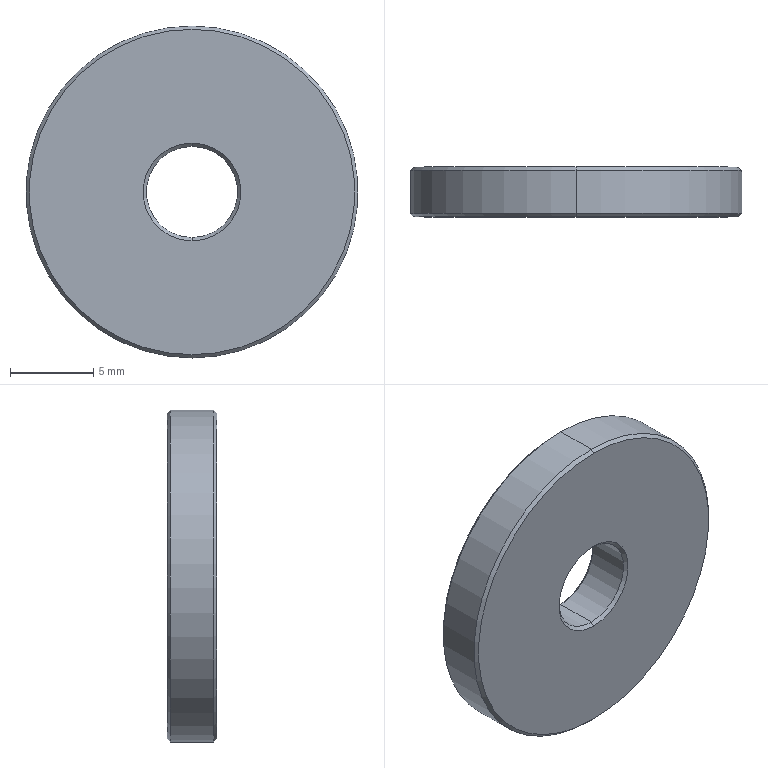Part | STEP file | 1 solid | 14 faces | box 20 x 3 x 20 mm | volume 867.998 mm3 | cone 8 | cylinder 4 | plane 2 | commonest cylinder face diameters 5.5 x2 20 x2
STEP:
#1=CARTESIAN_POINT('',(0.,0.,0.));
#2=DIRECTION('',(0.,0.,1.));
#3=DIRECTION('',(1.,0.,0.));
#4=AXIS2_PLACEMENT_3D('',#1,#2,#3);
#5=CARTESIAN_POINT('',(0.,2.8,2.75));
#6=VERTEX_POINT('',#5);
#7=CARTESIAN_POINT('',(0.,3.,2.95));
#8=VERTEX_POINT('',#7);
#9=CARTESIAN_POINT('',(0.,2.8,2.75));
#10=DIRECTION('',(0.,0.7071,0.7071));
#11=VECTOR('',#10,1.);
#12=LINE('',#9,#11);
#13=CARTESIAN_POINT('',(0.,2.8,0.));
#14=DIRECTION('',(0.,1.,0.));
#15=DIRECTION('',(0.,0.,1.));
#16=AXIS2_PLACEMENT_3D('',#13,#14,#15);
#17=CONICAL_SURFACE('',#16,2.75,0.7854);
#18=CARTESIAN_POINT('',(6.283,0.));
#19=DIRECTION('',(0.,1.));
#20=VECTOR('',#19,1.);
#21=LINE('',#18,#20);
#22=(GEOMETRIC_REPRESENTATION_CONTEXT(2)PARAMETRIC_REPRESENTATION_CONTEXT()REPRESENTATION_CONTEXT('',''));
#23=DEFINITIONAL_REPRESENTATION('',(#21),#22);
#24=PCURVE('',#17,#23);
#25=CARTESIAN_POINT('',(0.,2.8,0.));
#26=DIRECTION('',(0.,1.,0.));
#27=DIRECTION('',(0.,0.,1.));
#28=AXIS2_PLACEMENT_3D('',#25,#26,#27);
#29=CONICAL_SURFACE('',#28,2.75,0.7854);
#30=CARTESIAN_POINT('',(0.,0.));
#31=DIRECTION('',(0.,1.));
#32=VECTOR('',#31,1.);
#33=LINE('',#30,#32);
#34=(GEOMETRIC_REPRESENTATION_CONTEXT(2)PARAMETRIC_REPRESENTATION_CONTEXT()REPRESENTATION_CONTEXT('',''));
#35=DEFINITIONAL_REPRESENTATION('',(#33),#34);
#36=PCURVE('',#29,#35);
#37=SURFACE_CURVE('',#12,(#24,#36),.PCURVE_S1.);
#38=EDGE_CURVE('',#6,#8,#37,.T.);
#39=ORIENTED_EDGE('',*,*,#38,.T.);
#40=CARTESIAN_POINT('',(0.,3.,-2.95));
#41=VERTEX_POINT('',#40);
#42=CARTESIAN_POINT('',(0.,3.,0.));
#43=DIRECTION('',(0.,-1.,0.));
#44=DIRECTION('',(0.,0.,1.));
#45=AXIS2_PLACEMENT_3D('',#42,#43,#44);
#46=CIRCLE('',#45,2.95);
#47=CARTESIAN_POINT('',(6.283,0.2));
#48=DIRECTION('',(-1.,0.));
#49=VECTOR('',#48,1.);
#50=LINE('',#47,#49);
#51=(GEOMETRIC_REPRESENTATION_CONTEXT(2)PARAMETRIC_REPRESENTATION_CONTEXT()REPRESENTATION_CONTEXT('',''));
#52=DEFINITIONAL_REPRESENTATION('',(#50),#51);
#53=PCURVE('',#17,#52);
#54=CARTESIAN_POINT('',(0.,3.,0.));
#55=DIRECTION('',(0.,1.,0.));
#56=DIRECTION('',(0.,0.,1.));
#57=AXIS2_PLACEMENT_3D('',#54,#55,#56);
#58=PLANE('',#57);
#59=CARTESIAN_POINT('',(2.95,0.));
#60=CARTESIAN_POINT('',(2.95,-5.11));
#61=CARTESIAN_POINT('',(-1.475,-2.555));
#62=CARTESIAN_POINT('',(-5.9,0.));
#63=CARTESIAN_POINT('',(-1.475,2.555));
#64=CARTESIAN_POINT('',(2.95,5.11));
#65=CARTESIAN_POINT('',(2.95,0.));
#66=(BOUNDED_CURVE()B_SPLINE_CURVE(2,(#59,#60,#61,#62,#63,#64,#65),.UNSPECIFIED.,.T.,.F.)B_SPLINE_CURVE_WITH_KNOTS((1,2,2,2,2,1),(-2.094,0.,2.094,4.189,6.283,8.378),.UNSPECIFIED.)CURVE()GEOMETRIC_REPRESENTATION_ITEM()RATIONAL_B_SPLINE_CURVE((1.,0.5,1.,0.5,1.,0.5,1.))REPRESENTATION_ITEM(''));
#67=(GEOMETRIC_REPRESENTATION_CONTEXT(2)PARAMETRIC_REPRESENTATION_CONTEXT()REPRESENTATION_CONTEXT('',''));
#68=DEFINITIONAL_REPRESENTATION('',(#66),#67);
#69=PCURVE('',#58,#68);
#70=SURFACE_CURVE('',#46,(#53,#69),.PCURVE_S1.);
#71=EDGE_CURVE('',#8,#41,#70,.T.);
#72=ORIENTED_EDGE('',*,*,#71,.T.);
#73=CARTESIAN_POINT('',(0.,2.8,-2.75));
#74=VERTEX_POINT('',#73);
#75=CARTESIAN_POINT('',(0.,2.8,-2.75));
#76=DIRECTION('',(0.,0.7071,-0.7071));
#77=VECTOR('',#76,1.);
#78=LINE('',#75,#77);
#79=CARTESIAN_POINT('',(3.142,0.));
#80=DIRECTION('',(0.,1.));
#81=VECTOR('',#80,1.);
#82=LINE('',#79,#81);
#83=(GEOMETRIC_REPRESENTATION_CONTEXT(2)PARAMETRIC_REPRESENTATION_CONTEXT()REPRESENTATION_CONTEXT('',''));
#84=DEFINITIONAL_REPRESENTATION('',(#82),#83);
#85=PCURVE('',#17,#84);
#86=CARTESIAN_POINT('',(3.142,0.));
#87=DIRECTION('',(0.,1.));
#88=VECTOR('',#87,1.);
#89=LINE('',#86,#88);
#90=(GEOMETRIC_REPRESENTATION_CONTEXT(2)PARAMETRIC_REPRESENTATION_CONTEXT()REPRESENTATION_CONTEXT('',''));
#91=DEFINITIONAL_REPRESENTATION('',(#89),#90);
#92=PCURVE('',#29,#91);
#93=SURFACE_CURVE('',#78,(#85,#92),.PCURVE_S1.);
#94=EDGE_CURVE('',#74,#41,#93,.T.);
#95=ORIENTED_EDGE('',*,*,#94,.F.);
#96=CARTESIAN_POINT('',(0.,2.8,0.));
#97=DIRECTION('',(0.,1.,0.));
#98=DIRECTION('',(0.,0.,1.));
#99=AXIS2_PLACEMENT_3D('',#96,#97,#98);
#100=CIRCLE('',#99,2.75);
#101=CARTESIAN_POINT('',(0.,0.));
#102=DIRECTION('',(1.,0.));
#103=VECTOR('',#102,1.);
#104=LINE('',#101,#103);
#105=(GEOMETRIC_REPRESENTATION_CONTEXT(2)PARAMETRIC_REPRESENTATION_CONTEXT()REPRESENTATION_CONTEXT('',''));
#106=DEFINITIONAL_REPRESENTATION('',(#104),#105);
#107=PCURVE('',#17,#106);
#108=CARTESIAN_POINT('',(0.,3.,0.));
#109=DIRECTION('',(0.,-1.,0.));
#110=DIRECTION('',(0.,0.,-1.));
#111=AXIS2_PLACEMENT_3D('',#108,#109,#110);
#112=CYLINDRICAL_SURFACE('',#111,2.75);
#113=CARTESIAN_POINT('',(9.425,0.2));
#114=DIRECTION('',(-1.,0.));
#115=VECTOR('',#114,1.);
#116=LINE('',#113,#115);
#117=(GEOMETRIC_REPRESENTATION_CONTEXT(2)PARAMETRIC_REPRESENTATION_CONTEXT()REPRESENTATION_CONTEXT('',''));
#118=DEFINITIONAL_REPRESENTATION('',(#116),#117);
#119=PCURVE('',#112,#118);
#120=SURFACE_CURVE('',#100,(#107,#119),.PCURVE_S1.);
#121=EDGE_CURVE('',#74,#6,#120,.T.);
#122=ORIENTED_EDGE('',*,*,#121,.T.);
#123=EDGE_LOOP('',(#39,#72,#95,#122));
#124=FACE_BOUND('',#123,.F.);
#125=ADVANCED_FACE('',(#124),#17,.F.);
#126=CARTESIAN_POINT('',(0.,0.2,-2.75));
#127=VERTEX_POINT('',#126);
#128=CARTESIAN_POINT('',(0.,0.,-2.95));
#129=VERTEX_POINT('',#128);
#130=CARTESIAN_POINT('',(0.,0.,-2.95));
#131=DIRECTION('',(0.,-0.7071,-0.7071));
#132=VECTOR('',#131,1.);
#133=LINE('',#130,#132);
#134=CARTESIAN_POINT('',(0.,0.,0.));
#135=DIRECTION('',(0.,-1.,0.));
#136=DIRECTION('',(0.,0.,-1.));
#137=AXIS2_PLACEMENT_3D('',#134,#135,#136);
#138=CONICAL_SURFACE('',#137,2.95,0.7854);
#139=CARTESIAN_POINT('',(6.283,0.));
#140=DIRECTION('',(0.,1.));
#141=VECTOR('',#140,1.);
#142=LINE('',#139,#141);
#143=(GEOMETRIC_REPRESENTATION_CONTEXT(2)PARAMETRIC_REPRESENTATION_CONTEXT()REPRESENTATION_CONTEXT('',''));
#144=DEFINITIONAL_REPRESENTATION('',(#142),#143);
#145=PCURVE('',#138,#144);
#146=CARTESIAN_POINT('',(0.,0.,0.));
#147=DIRECTION('',(0.,-1.,0.));
#148=DIRECTION('',(0.,0.,-1.));
#149=AXIS2_PLACEMENT_3D('',#146,#147,#148);
#150=CONICAL_SURFACE('',#149,2.95,0.7854);
#151=CARTESIAN_POINT('',(0.,0.));
#152=DIRECTION('',(0.,1.));
#153=VECTOR('',#152,1.);
#154=LINE('',#151,#153);
#155=(GEOMETRIC_REPRESENTATION_CONTEXT(2)PARAMETRIC_REPRESENTATION_CONTEXT()REPRESENTATION_CONTEXT('',''));
#156=DEFINITIONAL_REPRESENTATION('',(#154),#155);
#157=PCURVE('',#150,#156);
#158=SURFACE_CURVE('',#133,(#145,#157),.PCURVE_S1.);
#159=EDGE_CURVE('',#127,#129,#158,.T.);
#160=ORIENTED_EDGE('',*,*,#159,.T.);
#161=CARTESIAN_POINT('',(0.,0.,2.95));
#162=VERTEX_POINT('',#161);
#163=CARTESIAN_POINT('',(0.,0.,0.));
#164=DIRECTION('',(0.,1.,0.));
#165=DIRECTION('',(0.,0.,1.));
#166=AXIS2_PLACEMENT_3D('',#163,#164,#165);
#167=CIRCLE('',#166,2.95);
#168=CARTESIAN_POINT('',(9.425,0.));
#169=DIRECTION('',(-1.,0.));
#170=VECTOR('',#169,1.);
#171=LINE('',#168,#170);
#172=(GEOMETRIC_REPRESENTATION_CONTEXT(2)PARAMETRIC_REPRESENTATION_CONTEXT()REPRESENTATION_CONTEXT('',''));
#173=DEFINITIONAL_REPRESENTATION('',(#171),#172);
#174=PCURVE('',#138,#173);
#175=CARTESIAN_POINT('',(0.,0.,0.));
#176=DIRECTION('',(0.,1.,0.));
#177=DIRECTION('',(0.,0.,1.));
#178=AXIS2_PLACEMENT_3D('',#175,#176,#177);
#179=PLANE('',#178);
#180=CARTESIAN_POINT('',(0.,0.));
#181=DIRECTION('',(1.,0.));
#182=AXIS2_PLACEMENT_2D('',#180,#181);
#183=CIRCLE('',#182,2.95);
#184=(GEOMETRIC_REPRESENTATION_CONTEXT(2)PARAMETRIC_REPRESENTATION_CONTEXT()REPRESENTATION_CONTEXT('',''));
#185=DEFINITIONAL_REPRESENTATION('',(#183),#184);
#186=PCURVE('',#179,#185);
#187=SURFACE_CURVE('',#167,(#174,#186),.PCURVE_S1.);
#188=EDGE_CURVE('',#129,#162,#187,.T.);
#189=ORIENTED_EDGE('',*,*,#188,.T.);
#190=CARTESIAN_POINT('',(0.,0.2,2.75));
#191=VERTEX_POINT('',#190);
#192=CARTESIAN_POINT('',(0.,0.,2.95));
#193=DIRECTION('',(0.,-0.7071,0.7071));
#194=VECTOR('',#193,1.);
#195=LINE('',#192,#194);
#196=CARTESIAN_POINT('',(3.142,0.));
#197=DIRECTION('',(0.,1.));
#198=VECTOR('',#197,1.);
#199=LINE('',#196,#198);
#200=(GEOMETRIC_REPRESENTATION_CONTEXT(2)PARAMETRIC_REPRESENTATION_CONTEXT()REPRESENTATION_CONTEXT('',''));
#201=DEFINITIONAL_REPRESENTATION('',(#199),#200);
#202=PCURVE('',#138,#201);
#203=CARTESIAN_POINT('',(3.142,0.));
#204=DIRECTION('',(0.,1.));
#205=VECTOR('',#204,1.);
#206=LINE('',#203,#205);
#207=(GEOMETRIC_REPRESENTATION_CONTEXT(2)PARAMETRIC_REPRESENTATION_CONTEXT()REPRESENTATION_CONTEXT('',''));
#208=DEFINITIONAL_REPRESENTATION('',(#206),#207);
#209=PCURVE('',#150,#208);
#210=SURFACE_CURVE('',#195,(#202,#209),.PCURVE_S1.);
#211=EDGE_CURVE('',#191,#162,#210,.T.);
#212=ORIENTED_EDGE('',*,*,#211,.F.);
#213=CARTESIAN_POINT('',(0.,0.2,0.));
#214=DIRECTION('',(0.,-1.,0.));
#215=DIRECTION('',(0.,0.,1.));
#216=AXIS2_PLACEMENT_3D('',#213,#214,#215);
#217=CIRCLE('',#216,2.75);
#218=CARTESIAN_POINT('',(3.142,-0.2));
#219=DIRECTION('',(1.,0.));
#220=VECTOR('',#219,1.);
#221=LINE('',#218,#220);
#222=(GEOMETRIC_REPRESENTATION_CONTEXT(2)PARAMETRIC_REPRESENTATION_CONTEXT()REPRESENTATION_CONTEXT('',''));
#223=DEFINITIONAL_REPRESENTATION('',(#221),#222);
#224=PCURVE('',#138,#223);
#225=CARTESIAN_POINT('',(3.142,2.8));
#226=DIRECTION('',(1.,0.));
#227=VECTOR('',#226,1.);
#228=LINE('',#225,#227);
#229=(GEOMETRIC_REPRESENTATION_CONTEXT(2)PARAMETRIC_REPRESENTATION_CONTEXT()REPRESENTATION_CONTEXT('',''));
#230=DEFINITIONAL_REPRESENTATION('',(#228),#229);
#231=PCURVE('',#112,#230);
#232=SURFACE_CURVE('',#217,(#224,#231),.PCURVE_S1.);
#233=EDGE_CURVE('',#191,#127,#232,.T.);
#234=ORIENTED_EDGE('',*,*,#233,.T.);
#235=EDGE_LOOP('',(#160,#189,#212,#234));
#236=FACE_BOUND('',#235,.F.);
#237=ADVANCED_FACE('',(#236),#138,.F.);
#238=CARTESIAN_POINT('',(0.,3.,9.8));
#239=VERTEX_POINT('',#238);
#240=CARTESIAN_POINT('',(0.,3.,-9.8));
#241=VERTEX_POINT('',#240);
#242=CARTESIAN_POINT('',(0.,3.,0.));
#243=DIRECTION('',(0.,1.,0.));
#244=DIRECTION('',(0.,0.,1.));
#245=AXIS2_PLACEMENT_3D('',#242,#243,#244);
#246=CIRCLE('',#245,9.8);
#247=CARTESIAN_POINT('',(0.,3.,0.));
#248=DIRECTION('',(0.,-1.,0.));
#249=DIRECTION('',(0.,0.,-1.));
#250=AXIS2_PLACEMENT_3D('',#247,#248,#249);
#251=CONICAL_SURFACE('',#250,9.8,0.7854);
#252=CARTESIAN_POINT('',(3.142,0.));
#253=DIRECTION('',(-1.,0.));
#254=VECTOR('',#253,1.);
#255=LINE('',#252,#254);
#256=(GEOMETRIC_REPRESENTATION_CONTEXT(2)PARAMETRIC_REPRESENTATION_CONTEXT()REPRESENTATION_CONTEXT('',''));
#257=DEFINITIONAL_REPRESENTATION('',(#255),#256);
#258=PCURVE('',#251,#257);
#259=CARTESIAN_POINT('',(0.,0.));
#260=DIRECTION('',(1.,0.));
#261=AXIS2_PLACEMENT_2D('',#259,#260);
#262=CIRCLE('',#261,9.8);
#263=(GEOMETRIC_REPRESENTATION_CONTEXT(2)PARAMETRIC_REPRESENTATION_CONTEXT()REPRESENTATION_CONTEXT('',''));
#264=DEFINITIONAL_REPRESENTATION('',(#262),#263);
#265=PCURVE('',#58,#264);
#266=SURFACE_CURVE('',#246,(#258,#265),.PCURVE_S1.);
#267=EDGE_CURVE('',#239,#241,#266,.T.);
#268=ORIENTED_EDGE('',*,*,#267,.F.);
#269=CARTESIAN_POINT('',(0.,2.8,10.));
#270=VERTEX_POINT('',#269);
#271=CARTESIAN_POINT('',(0.,3.,9.8));
#272=DIRECTION('',(0.,-0.7071,0.7071));
#273=VECTOR('',#272,1.);
#274=LINE('',#271,#273);
#275=CARTESIAN_POINT('',(3.142,0.));
#276=DIRECTION('',(0.,1.));
#277=VECTOR('',#276,1.);
#278=LINE('',#275,#277);
#279=(GEOMETRIC_REPRESENTATION_CONTEXT(2)PARAMETRIC_REPRESENTATION_CONTEXT()REPRESENTATION_CONTEXT('',''));
#280=DEFINITIONAL_REPRESENTATION('',(#278),#279);
#281=PCURVE('',#251,#280);
#282=CARTESIAN_POINT('',(0.,3.,0.));
#283=DIRECTION('',(0.,-1.,0.));
#284=DIRECTION('',(0.,0.,-1.));
#285=AXIS2_PLACEMENT_3D('',#282,#283,#284);
#286=CONICAL_SURFACE('',#285,9.8,0.7854);
#287=CARTESIAN_POINT('',(3.142,0.));
#288=DIRECTION('',(0.,1.));
#289=VECTOR('',#288,1.);
#290=LINE('',#287,#289);
#291=(GEOMETRIC_REPRESENTATION_CONTEXT(2)PARAMETRIC_REPRESENTATION_CONTEXT()REPRESENTATION_CONTEXT('',''));
#292=DEFINITIONAL_REPRESENTATION('',(#290),#291);
#293=PCURVE('',#286,#292);
#294=SURFACE_CURVE('',#274,(#281,#293),.PCURVE_S1.);
#295=EDGE_CURVE('',#239,#270,#294,.T.);
#296=ORIENTED_EDGE('',*,*,#295,.T.);
#297=CARTESIAN_POINT('',(0.,2.8,-10.));
#298=VERTEX_POINT('',#297);
#299=CARTESIAN_POINT('',(0.,2.8,0.));
#300=DIRECTION('',(0.,-1.,0.));
#301=DIRECTION('',(0.,0.,1.));
#302=AXIS2_PLACEMENT_3D('',#299,#300,#301);
#303=CIRCLE('',#302,10.);
#304=CARTESIAN_POINT('',(-3.142,0.2));
#305=DIRECTION('',(1.,0.));
#306=VECTOR('',#305,1.);
#307=LINE('',#304,#306);
#308=(GEOMETRIC_REPRESENTATION_CONTEXT(2)PARAMETRIC_REPRESENTATION_CONTEXT()REPRESENTATION_CONTEXT('',''));
#309=DEFINITIONAL_REPRESENTATION('',(#307),#308);
#310=PCURVE('',#251,#309);
#311=CARTESIAN_POINT('',(0.,3.,0.));
#312=DIRECTION('',(0.,-1.,0.));
#313=DIRECTION('',(0.,0.,-1.));
#314=AXIS2_PLACEMENT_3D('',#311,#312,#313);
#315=CYLINDRICAL_SURFACE('',#314,10.);
#316=CARTESIAN_POINT('',(-3.142,0.2));
#317=DIRECTION('',(1.,0.));
#318=VECTOR('',#317,1.);
#319=LINE('',#316,#318);
#320=(GEOMETRIC_REPRESENTATION_CONTEXT(2)PARAMETRIC_REPRESENTATION_CONTEXT()REPRESENTATION_CONTEXT('',''));
#321=DEFINITIONAL_REPRESENTATION('',(#319),#320);
#322=PCURVE('',#315,#321);
#323=SURFACE_CURVE('',#303,(#310,#322),.PCURVE_S1.);
#324=EDGE_CURVE('',#298,#270,#323,.T.);
#325=ORIENTED_EDGE('',*,*,#324,.F.);
#326=CARTESIAN_POINT('',(0.,3.,-9.8));
#327=DIRECTION('',(0.,-0.7071,-0.7071));
#328=VECTOR('',#327,1.);
#329=LINE('',#326,#328);
#330=CARTESIAN_POINT('',(0.,0.));
#331=DIRECTION('',(0.,1.));
#332=VECTOR('',#331,1.);
#333=LINE('',#330,#332);
#334=(GEOMETRIC_REPRESENTATION_CONTEXT(2)PARAMETRIC_REPRESENTATION_CONTEXT()REPRESENTATION_CONTEXT('',''));
#335=DEFINITIONAL_REPRESENTATION('',(#333),#334);
#336=PCURVE('',#251,#335);
#337=CARTESIAN_POINT('',(6.283,0.));
#338=DIRECTION('',(0.,1.));
#339=VECTOR('',#338,1.);
#340=LINE('',#337,#339);
#341=(GEOMETRIC_REPRESENTATION_CONTEXT(2)PARAMETRIC_REPRESENTATION_CONTEXT()REPRESENTATION_CONTEXT('',''));
#342=DEFINITIONAL_REPRESENTATION('',(#340),#341);
#343=PCURVE('',#286,#342);
#344=SURFACE_CURVE('',#329,(#336,#343),.PCURVE_S1.);
#345=EDGE_CURVE('',#241,#298,#344,.T.);
#346=ORIENTED_EDGE('',*,*,#345,.F.);
#347=EDGE_LOOP('',(#268,#296,#325,#346));
#348=FACE_BOUND('',#347,.T.);
#349=ADVANCED_FACE('',(#348),#251,.T.);
#350=CARTESIAN_POINT('',(0.,0.,-9.8));
#351=VERTEX_POINT('',#350);
#352=CARTESIAN_POINT('',(0.,0.,9.8));
#353=VERTEX_POINT('',#352);
#354=CARTESIAN_POINT('',(0.,0.,0.));
#355=DIRECTION('',(0.,-1.,0.));
#356=DIRECTION('',(0.,0.,1.));
#357=AXIS2_PLACEMENT_3D('',#354,#355,#356);
#358=CIRCLE('',#357,9.8);
#359=CARTESIAN_POINT('',(0.,0.2,0.));
#360=DIRECTION('',(0.,1.,0.));
#361=DIRECTION('',(0.,0.,1.));
#362=AXIS2_PLACEMENT_3D('',#359,#360,#361);
#363=CONICAL_SURFACE('',#362,10.,0.7854);
#364=CARTESIAN_POINT('',(6.283,-0.2));
#365=DIRECTION('',(-1.,0.));
#366=VECTOR('',#365,1.);
#367=LINE('',#364,#366);
#368=(GEOMETRIC_REPRESENTATION_CONTEXT(2)PARAMETRIC_REPRESENTATION_CONTEXT()REPRESENTATION_CONTEXT('',''));
#369=DEFINITIONAL_REPRESENTATION('',(#367),#368);
#370=PCURVE('',#363,#369);
#371=CARTESIAN_POINT('',(9.8,0.));
#372=CARTESIAN_POINT('',(9.8,-16.974));
#373=CARTESIAN_POINT('',(-4.9,-8.487));
#374=CARTESIAN_POINT('',(-19.6,0.));
#375=CARTESIAN_POINT('',(-4.9,8.487));
#376=CARTESIAN_POINT('',(9.8,16.974));
#377=CARTESIAN_POINT('',(9.8,0.));
#378=(BOUNDED_CURVE()B_SPLINE_CURVE(2,(#371,#372,#373,#374,#375,#376,#377),.UNSPECIFIED.,.T.,.F.)B_SPLINE_CURVE_WITH_KNOTS((1,2,2,2,2,1),(-2.094,0.,2.094,4.189,6.283,8.378),.UNSPECIFIED.)CURVE()GEOMETRIC_REPRESENTATION_ITEM()RATIONAL_B_SPLINE_CURVE((1.,0.5,1.,0.5,1.,0.5,1.))REPRESENTATION_ITEM(''));
#379=(GEOMETRIC_REPRESENTATION_CONTEXT(2)PARAMETRIC_REPRESENTATION_CONTEXT()REPRESENTATION_CONTEXT('',''));
#380=DEFINITIONAL_REPRESENTATION('',(#378),#379);
#381=PCURVE('',#179,#380);
#382=SURFACE_CURVE('',#358,(#370,#381),.PCURVE_S1.);
#383=EDGE_CURVE('',#351,#353,#382,.T.);
#384=ORIENTED_EDGE('',*,*,#383,.F.);
#385=CARTESIAN_POINT('',(0.,0.2,-10.));
#386=VERTEX_POINT('',#385);
#387=CARTESIAN_POINT('',(0.,0.2,-10.));
#388=DIRECTION('',(0.,0.7071,-0.7071));
#389=VECTOR('',#388,1.);
#390=LINE('',#387,#389);
#391=CARTESIAN_POINT('',(3.142,0.));
#392=DIRECTION('',(0.,1.));
#393=VECTOR('',#392,1.);
#394=LINE('',#391,#393);
#395=(GEOMETRIC_REPRESENTATION_CONTEXT(2)PARAMETRIC_REPRESENTATION_CONTEXT()REPRESENTATION_CONTEXT('',''));
#396=DEFINITIONAL_REPRESENTATION('',(#394),#395);
#397=PCURVE('',#363,#396);
#398=CARTESIAN_POINT('',(0.,0.2,0.));
#399=DIRECTION('',(0.,1.,0.));
#400=DIRECTION('',(0.,0.,1.));
#401=AXIS2_PLACEMENT_3D('',#398,#399,#400);
#402=CONICAL_SURFACE('',#401,10.,0.7854);
#403=CARTESIAN_POINT('',(3.142,0.));
#404=DIRECTION('',(0.,1.));
#405=VECTOR('',#404,1.);
#406=LINE('',#403,#405);
#407=(GEOMETRIC_REPRESENTATION_CONTEXT(2)PARAMETRIC_REPRESENTATION_CONTEXT()REPRESENTATION_CONTEXT('',''));
#408=DEFINITIONAL_REPRESENTATION('',(#406),#407);
#409=PCURVE('',#402,#408);
#410=SURFACE_CURVE('',#390,(#397,#409),.PCURVE_S1.);
#411=EDGE_CURVE('',#351,#386,#410,.T.);
#412=ORIENTED_EDGE('',*,*,#411,.T.);
#413=CARTESIAN_POINT('',(0.,0.2,10.));
#414=VERTEX_POINT('',#413);
#415=CARTESIAN_POINT('',(0.,0.2,0.));
#416=DIRECTION('',(0.,1.,0.));
#417=DIRECTION('',(0.,0.,1.));
#418=AXIS2_PLACEMENT_3D('',#415,#416,#417);
#419=CIRCLE('',#418,10.);
#420=CARTESIAN_POINT('',(0.,0.));
#421=DIRECTION('',(1.,0.));
#422=VECTOR('',#421,1.);
#423=LINE('',#420,#422);
#424=(GEOMETRIC_REPRESENTATION_CONTEXT(2)PARAMETRIC_REPRESENTATION_CONTEXT()REPRESENTATION_CONTEXT('',''));
#425=DEFINITIONAL_REPRESENTATION('',(#423),#424);
#426=PCURVE('',#363,#425);
#427=CARTESIAN_POINT('',(3.142,2.8));
#428=DIRECTION('',(-1.,0.));
#429=VECTOR('',#428,1.);
#430=LINE('',#427,#429);
#431=(GEOMETRIC_REPRESENTATION_CONTEXT(2)PARAMETRIC_REPRESENTATION_CONTEXT()REPRESENTATION_CONTEXT('',''));
#432=DEFINITIONAL_REPRESENTATION('',(#430),#431);
#433=PCURVE('',#315,#432);
#434=SURFACE_CURVE('',#419,(#426,#433),.PCURVE_S1.);
#435=EDGE_CURVE('',#414,#386,#434,.T.);
#436=ORIENTED_EDGE('',*,*,#435,.F.);
#437=CARTESIAN_POINT('',(0.,0.2,10.));
#438=DIRECTION('',(0.,0.7071,0.7071));
#439=VECTOR('',#438,1.);
#440=LINE('',#437,#439);
#441=CARTESIAN_POINT('',(0.,0.));
#442=DIRECTION('',(0.,1.));
#443=VECTOR('',#442,1.);
#444=LINE('',#441,#443);
#445=(GEOMETRIC_REPRESENTATION_CONTEXT(2)PARAMETRIC_REPRESENTATION_CONTEXT()REPRESENTATION_CONTEXT('',''));
#446=DEFINITIONAL_REPRESENTATION('',(#444),#445);
#447=PCURVE('',#363,#446);
#448=CARTESIAN_POINT('',(6.283,0.));
#449=DIRECTION('',(0.,1.));
#450=VECTOR('',#449,1.);
#451=LINE('',#448,#450);
#452=(GEOMETRIC_REPRESENTATION_CONTEXT(2)PARAMETRIC_REPRESENTATION_CONTEXT()REPRESENTATION_CONTEXT('',''));
#453=DEFINITIONAL_REPRESENTATION('',(#451),#452);
#454=PCURVE('',#402,#453);
#455=SURFACE_CURVE('',#440,(#447,#454),.PCURVE_S1.);
#456=EDGE_CURVE('',#353,#414,#455,.T.);
#457=ORIENTED_EDGE('',*,*,#456,.F.);
#458=EDGE_LOOP('',(#384,#412,#436,#457));
#459=FACE_BOUND('',#458,.T.);
#460=ADVANCED_FACE('',(#459),#363,.T.);
#461=CARTESIAN_POINT('',(0.,3.,-2.75));
#462=DIRECTION('',(0.,-1.,0.));
#463=VECTOR('',#462,1.);
#464=LINE('',#461,#463);
#465=CARTESIAN_POINT('',(6.283,0.));
#466=DIRECTION('',(0.,1.));
#467=VECTOR('',#466,1.);
#468=LINE('',#465,#467);
#469=(GEOMETRIC_REPRESENTATION_CONTEXT(2)PARAMETRIC_REPRESENTATION_CONTEXT()REPRESENTATION_CONTEXT('',''));
#470=DEFINITIONAL_REPRESENTATION('',(#468),#469);
#471=PCURVE('',#112,#470);
#472=CARTESIAN_POINT('',(0.,3.,0.));
#473=DIRECTION('',(0.,-1.,0.));
#474=DIRECTION('',(0.,0.,-1.));
#475=AXIS2_PLACEMENT_3D('',#472,#473,#474);
#476=CYLINDRICAL_SURFACE('',#475,2.75);
#477=CARTESIAN_POINT('',(0.,0.));
#478=DIRECTION('',(0.,1.));
#479=VECTOR('',#478,1.);
#480=LINE('',#477,#479);
#481=(GEOMETRIC_REPRESENTATION_CONTEXT(2)PARAMETRIC_REPRESENTATION_CONTEXT()REPRESENTATION_CONTEXT('',''));
#482=DEFINITIONAL_REPRESENTATION('',(#480),#481);
#483=PCURVE('',#476,#482);
#484=SURFACE_CURVE('',#464,(#471,#483),.PCURVE_S1.);
#485=EDGE_CURVE('',#74,#127,#484,.T.);
#486=ORIENTED_EDGE('',*,*,#485,.T.);
#487=ORIENTED_EDGE('',*,*,#233,.F.);
#488=CARTESIAN_POINT('',(0.,3.,2.75));
#489=DIRECTION('',(0.,-1.,0.));
#490=VECTOR('',#489,1.);
#491=LINE('',#488,#490);
#492=CARTESIAN_POINT('',(3.142,0.));
#493=DIRECTION('',(0.,1.));
#494=VECTOR('',#493,1.);
#495=LINE('',#492,#494);
#496=(GEOMETRIC_REPRESENTATION_CONTEXT(2)PARAMETRIC_REPRESENTATION_CONTEXT()REPRESENTATION_CONTEXT('',''));
#497=DEFINITIONAL_REPRESENTATION('',(#495),#496);
#498=PCURVE('',#112,#497);
#499=CARTESIAN_POINT('',(3.142,0.));
#500=DIRECTION('',(0.,1.));
#501=VECTOR('',#500,1.);
#502=LINE('',#499,#501);
#503=(GEOMETRIC_REPRESENTATION_CONTEXT(2)PARAMETRIC_REPRESENTATION_CONTEXT()REPRESENTATION_CONTEXT('',''));
#504=DEFINITIONAL_REPRESENTATION('',(#502),#503);
#505=PCURVE('',#476,#504);
#506=SURFACE_CURVE('',#491,(#498,#505),.PCURVE_S1.);
#507=EDGE_CURVE('',#6,#191,#506,.T.);
#508=ORIENTED_EDGE('',*,*,#507,.F.);
#509=ORIENTED_EDGE('',*,*,#121,.F.);
#510=EDGE_LOOP('',(#486,#487,#508,#509));
#511=FACE_BOUND('',#510,.F.);
#512=ADVANCED_FACE('',(#511),#112,.F.);
#513=ORIENTED_EDGE('',*,*,#324,.T.);
#514=CARTESIAN_POINT('',(0.,3.,10.));
#515=DIRECTION('',(0.,-1.,0.));
#516=VECTOR('',#515,1.);
#517=LINE('',#514,#516);
#518=CARTESIAN_POINT('',(3.142,0.));
#519=DIRECTION('',(0.,1.));
#520=VECTOR('',#519,1.);
#521=LINE('',#518,#520);
#522=(GEOMETRIC_REPRESENTATION_CONTEXT(2)PARAMETRIC_REPRESENTATION_CONTEXT()REPRESENTATION_CONTEXT('',''));
#523=DEFINITIONAL_REPRESENTATION('',(#521),#522);
#524=PCURVE('',#315,#523);
#525=CARTESIAN_POINT('',(0.,3.,0.));
#526=DIRECTION('',(0.,-1.,0.));
#527=DIRECTION('',(0.,0.,-1.));
#528=AXIS2_PLACEMENT_3D('',#525,#526,#527);
#529=CYLINDRICAL_SURFACE('',#528,10.);
#530=CARTESIAN_POINT('',(3.142,0.));
#531=DIRECTION('',(0.,1.));
#532=VECTOR('',#531,1.);
#533=LINE('',#530,#532);
#534=(GEOMETRIC_REPRESENTATION_CONTEXT(2)PARAMETRIC_REPRESENTATION_CONTEXT()REPRESENTATION_CONTEXT('',''));
#535=DEFINITIONAL_REPRESENTATION('',(#533),#534);
#536=PCURVE('',#529,#535);
#537=SURFACE_CURVE('',#517,(#524,#536),.PCURVE_S1.);
#538=EDGE_CURVE('',#270,#414,#537,.T.);
#539=ORIENTED_EDGE('',*,*,#538,.T.);
#540=ORIENTED_EDGE('',*,*,#435,.T.);
#541=CARTESIAN_POINT('',(0.,3.,-10.));
#542=DIRECTION('',(0.,-1.,0.));
#543=VECTOR('',#542,1.);
#544=LINE('',#541,#543);
#545=CARTESIAN_POINT('',(0.,0.));
#546=DIRECTION('',(0.,1.));
#547=VECTOR('',#546,1.);
#548=LINE('',#545,#547);
#549=(GEOMETRIC_REPRESENTATION_CONTEXT(2)PARAMETRIC_REPRESENTATION_CONTEXT()REPRESENTATION_CONTEXT('',''));
#550=DEFINITIONAL_REPRESENTATION('',(#548),#549);
#551=PCURVE('',#315,#550);
#552=CARTESIAN_POINT('',(6.283,0.));
#553=DIRECTION('',(0.,1.));
#554=VECTOR('',#553,1.);
#555=LINE('',#552,#554);
#556=(GEOMETRIC_REPRESENTATION_CONTEXT(2)PARAMETRIC_REPRESENTATION_CONTEXT()REPRESENTATION_CONTEXT('',''));
#557=DEFINITIONAL_REPRESENTATION('',(#555),#556);
#558=PCURVE('',#529,#557);
#559=SURFACE_CURVE('',#544,(#551,#558),.PCURVE_S1.);
#560=EDGE_CURVE('',#298,#386,#559,.T.);
#561=ORIENTED_EDGE('',*,*,#560,.F.);
#562=EDGE_LOOP('',(#513,#539,#540,#561));
#563=FACE_BOUND('',#562,.T.);
#564=ADVANCED_FACE('',(#563),#315,.T.);
#565=CARTESIAN_POINT('',(0.,3.,0.));
#566=DIRECTION('',(0.,1.,0.));
#567=DIRECTION('',(0.,0.,1.));
#568=AXIS2_PLACEMENT_3D('',#565,#566,#567);
#569=CIRCLE('',#568,9.8);
#570=CARTESIAN_POINT('',(0.,0.));
#571=DIRECTION('',(1.,0.));
#572=AXIS2_PLACEMENT_2D('',#570,#571);
#573=CIRCLE('',#572,9.8);
#574=(GEOMETRIC_REPRESENTATION_CONTEXT(2)PARAMETRIC_REPRESENTATION_CONTEXT()REPRESENTATION_CONTEXT('',''));
#575=DEFINITIONAL_REPRESENTATION('',(#573),#574);
#576=PCURVE('',#58,#575);
#577=CARTESIAN_POINT('',(9.425,0.));
#578=DIRECTION('',(-1.,0.));
#579=VECTOR('',#578,1.);
#580=LINE('',#577,#579);
#581=(GEOMETRIC_REPRESENTATION_CONTEXT(2)PARAMETRIC_REPRESENTATION_CONTEXT()REPRESENTATION_CONTEXT('',''));
#582=DEFINITIONAL_REPRESENTATION('',(#580),#581);
#583=PCURVE('',#286,#582);
#584=SURFACE_CURVE('',#569,(#576,#583),.PCURVE_S1.);
#585=EDGE_CURVE('',#241,#239,#584,.T.);
#586=ORIENTED_EDGE('',*,*,#585,.T.);
#587=ORIENTED_EDGE('',*,*,#267,.T.);
#588=EDGE_LOOP('',(#586,#587));
#589=FACE_BOUND('',#588,.T.);
#590=ORIENTED_EDGE('',*,*,#71,.T.);
#591=CARTESIAN_POINT('',(0.,3.,0.));
#592=DIRECTION('',(0.,-1.,0.));
#593=DIRECTION('',(0.,0.,1.));
#594=AXIS2_PLACEMENT_3D('',#591,#592,#593);
#595=CIRCLE('',#594,2.95);
#596=CARTESIAN_POINT('',(2.95,0.));
#597=CARTESIAN_POINT('',(2.95,-5.11));
#598=CARTESIAN_POINT('',(-1.475,-2.555));
#599=CARTESIAN_POINT('',(-5.9,0.));
#600=CARTESIAN_POINT('',(-1.475,2.555));
#601=CARTESIAN_POINT('',(2.95,5.11));
#602=CARTESIAN_POINT('',(2.95,0.));
#603=(BOUNDED_CURVE()B_SPLINE_CURVE(2,(#596,#597,#598,#599,#600,#601,#602),.UNSPECIFIED.,.T.,.F.)B_SPLINE_CURVE_WITH_KNOTS((1,2,2,2,2,1),(-2.094,0.,2.094,4.189,6.283,8.378),.UNSPECIFIED.)CURVE()GEOMETRIC_REPRESENTATION_ITEM()RATIONAL_B_SPLINE_CURVE((1.,0.5,1.,0.5,1.,0.5,1.))REPRESENTATION_ITEM(''));
#604=(GEOMETRIC_REPRESENTATION_CONTEXT(2)PARAMETRIC_REPRESENTATION_CONTEXT()REPRESENTATION_CONTEXT('',''));
#605=DEFINITIONAL_REPRESENTATION('',(#603),#604);
#606=PCURVE('',#58,#605);
#607=CARTESIAN_POINT('',(6.283,0.2));
#608=DIRECTION('',(-1.,0.));
#609=VECTOR('',#608,1.);
#610=LINE('',#607,#609);
#611=(GEOMETRIC_REPRESENTATION_CONTEXT(2)PARAMETRIC_REPRESENTATION_CONTEXT()REPRESENTATION_CONTEXT('',''));
#612=DEFINITIONAL_REPRESENTATION('',(#610),#611);
#613=PCURVE('',#29,#612);
#614=SURFACE_CURVE('',#595,(#606,#613),.PCURVE_S1.);
#615=EDGE_CURVE('',#41,#8,#614,.T.);
#616=ORIENTED_EDGE('',*,*,#615,.T.);
#617=EDGE_LOOP('',(#590,#616));
#618=FACE_BOUND('',#617,.T.);
#619=ADVANCED_FACE('',(#589,#618),#58,.T.);
#620=CARTESIAN_POINT('',(0.,0.,0.));
#621=DIRECTION('',(0.,-1.,0.));
#622=DIRECTION('',(0.,0.,1.));
#623=AXIS2_PLACEMENT_3D('',#620,#621,#622);
#624=CIRCLE('',#623,9.8);
#625=CARTESIAN_POINT('',(9.8,0.));
#626=CARTESIAN_POINT('',(9.8,-16.974));
#627=CARTESIAN_POINT('',(-4.9,-8.487));
#628=CARTESIAN_POINT('',(-19.6,0.));
#629=CARTESIAN_POINT('',(-4.9,8.487));
#630=CARTESIAN_POINT('',(9.8,16.974));
#631=CARTESIAN_POINT('',(9.8,0.));
#632=(BOUNDED_CURVE()B_SPLINE_CURVE(2,(#625,#626,#627,#628,#629,#630,#631),.UNSPECIFIED.,.T.,.F.)B_SPLINE_CURVE_WITH_KNOTS((1,2,2,2,2,1),(-2.094,0.,2.094,4.189,6.283,8.378),.UNSPECIFIED.)CURVE()GEOMETRIC_REPRESENTATION_ITEM()RATIONAL_B_SPLINE_CURVE((1.,0.5,1.,0.5,1.,0.5,1.))REPRESENTATION_ITEM(''));
#633=(GEOMETRIC_REPRESENTATION_CONTEXT(2)PARAMETRIC_REPRESENTATION_CONTEXT()REPRESENTATION_CONTEXT('',''));
#634=DEFINITIONAL_REPRESENTATION('',(#632),#633);
#635=PCURVE('',#179,#634);
#636=CARTESIAN_POINT('',(6.283,-0.2));
#637=DIRECTION('',(-1.,0.));
#638=VECTOR('',#637,1.);
#639=LINE('',#636,#638);
#640=(GEOMETRIC_REPRESENTATION_CONTEXT(2)PARAMETRIC_REPRESENTATION_CONTEXT()REPRESENTATION_CONTEXT('',''));
#641=DEFINITIONAL_REPRESENTATION('',(#639),#640);
#642=PCURVE('',#402,#641);
#643=SURFACE_CURVE('',#624,(#635,#642),.PCURVE_S1.);
#644=EDGE_CURVE('',#353,#351,#643,.T.);
#645=ORIENTED_EDGE('',*,*,#644,.T.);
#646=ORIENTED_EDGE('',*,*,#383,.T.);
#647=EDGE_LOOP('',(#645,#646));
#648=FACE_BOUND('',#647,.T.);
#649=ORIENTED_EDGE('',*,*,#188,.T.);
#650=CARTESIAN_POINT('',(0.,0.,0.));
#651=DIRECTION('',(0.,1.,0.));
#652=DIRECTION('',(0.,0.,1.));
#653=AXIS2_PLACEMENT_3D('',#650,#651,#652);
#654=CIRCLE('',#653,2.95);
#655=CARTESIAN_POINT('',(0.,0.));
#656=DIRECTION('',(1.,0.));
#657=AXIS2_PLACEMENT_2D('',#655,#656);
#658=CIRCLE('',#657,2.95);
#659=(GEOMETRIC_REPRESENTATION_CONTEXT(2)PARAMETRIC_REPRESENTATION_CONTEXT()REPRESENTATION_CONTEXT('',''));
#660=DEFINITIONAL_REPRESENTATION('',(#658),#659);
#661=PCURVE('',#179,#660);
#662=CARTESIAN_POINT('',(3.142,0.));
#663=DIRECTION('',(-1.,0.));
#664=VECTOR('',#663,1.);
#665=LINE('',#662,#664);
#666=(GEOMETRIC_REPRESENTATION_CONTEXT(2)PARAMETRIC_REPRESENTATION_CONTEXT()REPRESENTATION_CONTEXT('',''));
#667=DEFINITIONAL_REPRESENTATION('',(#665),#666);
#668=PCURVE('',#150,#667);
#669=SURFACE_CURVE('',#654,(#661,#668),.PCURVE_S1.);
#670=EDGE_CURVE('',#162,#129,#669,.T.);
#671=ORIENTED_EDGE('',*,*,#670,.T.);
#672=EDGE_LOOP('',(#649,#671));
#673=FACE_BOUND('',#672,.T.);
#674=ADVANCED_FACE('',(#648,#673),#179,.F.);
#675=ORIENTED_EDGE('',*,*,#538,.F.);
#676=CARTESIAN_POINT('',(0.,2.8,0.));
#677=DIRECTION('',(0.,-1.,0.));
#678=DIRECTION('',(0.,0.,1.));
#679=AXIS2_PLACEMENT_3D('',#676,#677,#678);
#680=CIRCLE('',#679,10.);
#681=CARTESIAN_POINT('',(3.142,0.2));
#682=DIRECTION('',(1.,0.));
#683=VECTOR('',#682,1.);
#684=LINE('',#681,#683);
#685=(GEOMETRIC_REPRESENTATION_CONTEXT(2)PARAMETRIC_REPRESENTATION_CONTEXT()REPRESENTATION_CONTEXT('',''));
#686=DEFINITIONAL_REPRESENTATION('',(#684),#685);
#687=PCURVE('',#529,#686);
#688=CARTESIAN_POINT('',(3.142,0.2));
#689=DIRECTION('',(1.,0.));
#690=VECTOR('',#689,1.);
#691=LINE('',#688,#690);
#692=(GEOMETRIC_REPRESENTATION_CONTEXT(2)PARAMETRIC_REPRESENTATION_CONTEXT()REPRESENTATION_CONTEXT('',''));
#693=DEFINITIONAL_REPRESENTATION('',(#691),#692);
#694=PCURVE('',#286,#693);
#695=SURFACE_CURVE('',#680,(#687,#694),.PCURVE_S1.);
#696=EDGE_CURVE('',#270,#298,#695,.T.);
#697=ORIENTED_EDGE('',*,*,#696,.T.);
#698=ORIENTED_EDGE('',*,*,#560,.T.);
#699=CARTESIAN_POINT('',(0.,0.2,0.));
#700=DIRECTION('',(0.,1.,0.));
#701=DIRECTION('',(0.,0.,1.));
#702=AXIS2_PLACEMENT_3D('',#699,#700,#701);
#703=CIRCLE('',#702,10.);
#704=CARTESIAN_POINT('',(9.425,2.8));
#705=DIRECTION('',(-1.,0.));
#706=VECTOR('',#705,1.);
#707=LINE('',#704,#706);
#708=(GEOMETRIC_REPRESENTATION_CONTEXT(2)PARAMETRIC_REPRESENTATION_CONTEXT()REPRESENTATION_CONTEXT('',''));
#709=DEFINITIONAL_REPRESENTATION('',(#707),#708);
#710=PCURVE('',#529,#709);
#711=CARTESIAN_POINT('',(0.,0.));
#712=DIRECTION('',(1.,0.));
#713=VECTOR('',#712,1.);
#714=LINE('',#711,#713);
#715=(GEOMETRIC_REPRESENTATION_CONTEXT(2)PARAMETRIC_REPRESENTATION_CONTEXT()REPRESENTATION_CONTEXT('',''));
#716=DEFINITIONAL_REPRESENTATION('',(#714),#715);
#717=PCURVE('',#402,#716);
#718=SURFACE_CURVE('',#703,(#710,#717),.PCURVE_S1.);
#719=EDGE_CURVE('',#386,#414,#718,.T.);
#720=ORIENTED_EDGE('',*,*,#719,.T.);
#721=EDGE_LOOP('',(#675,#697,#698,#720));
#722=FACE_BOUND('',#721,.T.);
#723=ADVANCED_FACE('',(#722),#529,.T.);
#724=CARTESIAN_POINT('',(0.,0.2,0.));
#725=DIRECTION('',(0.,-1.,0.));
#726=DIRECTION('',(0.,0.,1.));
#727=AXIS2_PLACEMENT_3D('',#724,#725,#726);
#728=CIRCLE('',#727,2.75);
#729=CARTESIAN_POINT('',(-3.142,2.8));
#730=DIRECTION('',(1.,0.));
#731=VECTOR('',#730,1.);
#732=LINE('',#729,#731);
#733=(GEOMETRIC_REPRESENTATION_CONTEXT(2)PARAMETRIC_REPRESENTATION_CONTEXT()REPRESENTATION_CONTEXT('',''));
#734=DEFINITIONAL_REPRESENTATION('',(#732),#733);
#735=PCURVE('',#476,#734);
#736=CARTESIAN_POINT('',(-3.142,-0.2));
#737=DIRECTION('',(1.,0.));
#738=VECTOR('',#737,1.);
#739=LINE('',#736,#738);
#740=(GEOMETRIC_REPRESENTATION_CONTEXT(2)PARAMETRIC_REPRESENTATION_CONTEXT()REPRESENTATION_CONTEXT('',''));
#741=DEFINITIONAL_REPRESENTATION('',(#739),#740);
#742=PCURVE('',#150,#741);
#743=SURFACE_CURVE('',#728,(#735,#742),.PCURVE_S1.);
#744=EDGE_CURVE('',#127,#191,#743,.T.);
#745=ORIENTED_EDGE('',*,*,#744,.F.);
#746=ORIENTED_EDGE('',*,*,#485,.F.);
#747=CARTESIAN_POINT('',(0.,2.8,0.));
#748=DIRECTION('',(0.,1.,0.));
#749=DIRECTION('',(0.,0.,1.));
#750=AXIS2_PLACEMENT_3D('',#747,#748,#749);
#751=CIRCLE('',#750,2.75);
#752=CARTESIAN_POINT('',(3.142,0.2));
#753=DIRECTION('',(-1.,0.));
#754=VECTOR('',#753,1.);
#755=LINE('',#752,#754);
#756=(GEOMETRIC_REPRESENTATION_CONTEXT(2)PARAMETRIC_REPRESENTATION_CONTEXT()REPRESENTATION_CONTEXT('',''));
#757=DEFINITIONAL_REPRESENTATION('',(#755),#756);
#758=PCURVE('',#476,#757);
#759=CARTESIAN_POINT('',(0.,0.));
#760=DIRECTION('',(1.,0.));
#761=VECTOR('',#760,1.);
#762=LINE('',#759,#761);
#763=(GEOMETRIC_REPRESENTATION_CONTEXT(2)PARAMETRIC_REPRESENTATION_CONTEXT()REPRESENTATION_CONTEXT('',''));
#764=DEFINITIONAL_REPRESENTATION('',(#762),#763);
#765=PCURVE('',#29,#764);
#766=SURFACE_CURVE('',#751,(#758,#765),.PCURVE_S1.);
#767=EDGE_CURVE('',#6,#74,#766,.T.);
#768=ORIENTED_EDGE('',*,*,#767,.F.);
#769=ORIENTED_EDGE('',*,*,#507,.T.);
#770=EDGE_LOOP('',(#745,#746,#768,#769));
#771=FACE_BOUND('',#770,.F.);
#772=ADVANCED_FACE('',(#771),#476,.F.);
#773=ORIENTED_EDGE('',*,*,#411,.F.);
#774=ORIENTED_EDGE('',*,*,#644,.F.);
#775=ORIENTED_EDGE('',*,*,#456,.T.);
#776=ORIENTED_EDGE('',*,*,#719,.F.);
#777=EDGE_LOOP('',(#773,#774,#775,#776));
#778=FACE_BOUND('',#777,.T.);
#779=ADVANCED_FACE('',(#778),#402,.T.);
#780=ORIENTED_EDGE('',*,*,#295,.F.);
#781=ORIENTED_EDGE('',*,*,#585,.F.);
#782=ORIENTED_EDGE('',*,*,#345,.T.);
#783=ORIENTED_EDGE('',*,*,#696,.F.);
#784=EDGE_LOOP('',(#780,#781,#782,#783));
#785=FACE_BOUND('',#784,.T.);
#786=ADVANCED_FACE('',(#785),#286,.T.);
#787=ORIENTED_EDGE('',*,*,#670,.T.);
#788=ORIENTED_EDGE('',*,*,#159,.F.);
#789=ORIENTED_EDGE('',*,*,#744,.T.);
#790=ORIENTED_EDGE('',*,*,#211,.T.);
#791=EDGE_LOOP('',(#787,#788,#789,#790));
#792=FACE_BOUND('',#791,.F.);
#793=ADVANCED_FACE('',(#792),#150,.F.);
#794=ORIENTED_EDGE('',*,*,#615,.T.);
#795=ORIENTED_EDGE('',*,*,#38,.F.);
#796=ORIENTED_EDGE('',*,*,#767,.T.);
#797=ORIENTED_EDGE('',*,*,#94,.T.);
#798=EDGE_LOOP('',(#794,#795,#796,#797));
#799=FACE_BOUND('',#798,.F.);
#800=ADVANCED_FACE('',(#799),#29,.F.);
#801=CLOSED_SHELL('',(#125,#237,#349,#460,#512,#564,#619,#674,#723,#772,#779,#786,#793,#800));
#802=MANIFOLD_SOLID_BREP('',#801);
#803=(LENGTH_UNIT()NAMED_UNIT(*)SI_UNIT(.MILLI.,.METRE.));
#804=UNCERTAINTY_MEASURE_WITH_UNIT(LENGTH_MEASURE(0.0000001),#803,'','');
#805=(NAMED_UNIT(*)PLANE_ANGLE_UNIT()SI_UNIT($,.RADIAN.));
#806=(NAMED_UNIT(*)SI_UNIT($,.STERADIAN.)SOLID_ANGLE_UNIT());
#807=(GEOMETRIC_REPRESENTATION_CONTEXT(3)GLOBAL_UNCERTAINTY_ASSIGNED_CONTEXT((#804))GLOBAL_UNIT_ASSIGNED_CONTEXT((#803,#805,#806))REPRESENTATION_CONTEXT('',''));
#808=ADVANCED_BREP_SHAPE_REPRESENTATION('',(#4,#802),#807);